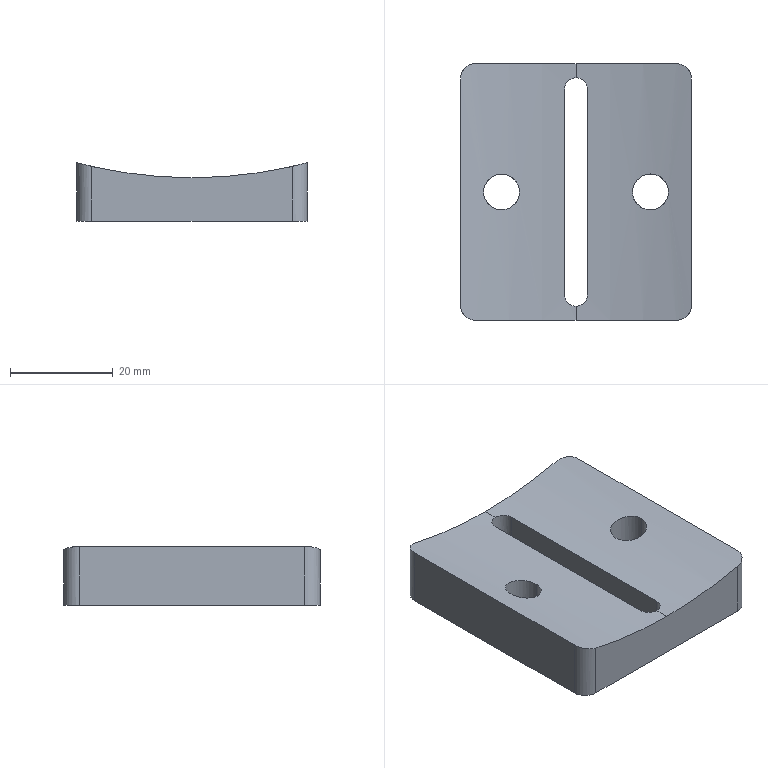Part | SolidWorks | features ICE 2, Extrusion 1, Fillet 1, HoleWzd 1 | 1 solid | 24 faces | box 45 x 50 x 11.442 mm | volume 18116 mm3 | cylinder 14 | plane 10 | commonest cylinder face diameters 6 x4 7 x4 4.5 x2 8 x2 175 x2
STEP:
#1=CARTESIAN_POINT('',(18.,25.,-85.629));
#2=VERTEX_POINT('',#1);
#3=CARTESIAN_POINT('',(11.,25.,-86.806));
#4=VERTEX_POINT('',#3);
#5=CARTESIAN_POINT('',(18.,25.,-85.629));
#6=CARTESIAN_POINT('',(18.,24.77,-85.629));
#7=CARTESIAN_POINT('',(17.978,24.541,-85.633));
#8=CARTESIAN_POINT('',(17.887,24.087,-85.652));
#9=CARTESIAN_POINT('',(17.819,23.865,-85.666));
#10=CARTESIAN_POINT('',(17.643,23.443,-85.703));
#11=CARTESIAN_POINT('',(17.533,23.239,-85.725));
#12=CARTESIAN_POINT('',(17.276,22.856,-85.778));
#13=CARTESIAN_POINT('',(17.131,22.681,-85.807));
#14=CARTESIAN_POINT('',(16.808,22.359,-85.871));
#15=CARTESIAN_POINT('',(16.628,22.212,-85.906));
#16=CARTESIAN_POINT('',(16.25,21.96,-85.978));
#17=CARTESIAN_POINT('',(16.05,21.854,-86.016));
#18=CARTESIAN_POINT('',(15.629,21.679,-86.093));
#19=CARTESIAN_POINT('',(15.409,21.612,-86.133));
#20=CARTESIAN_POINT('',(14.965,21.524,-86.211));
#21=CARTESIAN_POINT('',(14.739,21.501,-86.25));
#22=CARTESIAN_POINT('',(14.28,21.499,-86.327));
#23=CARTESIAN_POINT('',(14.054,21.521,-86.364));
#24=CARTESIAN_POINT('',(13.609,21.608,-86.436));
#25=CARTESIAN_POINT('',(13.388,21.674,-86.47));
#26=CARTESIAN_POINT('',(12.964,21.847,-86.535));
#27=CARTESIAN_POINT('',(12.763,21.953,-86.564));
#28=CARTESIAN_POINT('',(12.381,22.205,-86.62));
#29=CARTESIAN_POINT('',(12.2,22.352,-86.645));
#30=CARTESIAN_POINT('',(11.875,22.674,-86.691));
#31=CARTESIAN_POINT('',(11.729,22.85,-86.71));
#32=CARTESIAN_POINT('',(11.47,23.232,-86.745));
#33=CARTESIAN_POINT('',(11.36,23.437,-86.76));
#34=CARTESIAN_POINT('',(11.094,24.072,-86.794));
#35=CARTESIAN_POINT('',(11.,24.534,-86.806));
#36=CARTESIAN_POINT('',(11.,25.,-86.806));
#37=B_SPLINE_CURVE_WITH_KNOTS('',3,(#5,#6,#7,#8,#9,#10,#11,#12,#13,#14,#15,#16,#17,#18,#19,#20,#21,#22,#23,#24,#25,#26,#27,#28,#29,#30,#31,#32,#33,#34,#35,#36),.UNSPECIFIED.,.F.,.F.,(4,2,2,2,2,2,2,2,2,2,2,2,2,2,2,4),(0.01102,0.01171,0.0124,0.01309,0.01378,0.01447,0.01515,0.01584,0.01653,0.01722,0.01791,0.0186,0.01929,0.01997,0.02066,0.02204),.UNSPECIFIED.);
#38=EDGE_CURVE('',#2,#4,#37,.T.);
#39=ORIENTED_EDGE('',*,*,#38,.F.);
#40=CARTESIAN_POINT('',(18.,25.,-96.));
#41=VERTEX_POINT('',#40);
#42=CARTESIAN_POINT('',(18.,25.,-96.));
#43=DIRECTION('',(0.,0.,-1.));
#44=VECTOR('',#43,1000.);
#45=LINE('',#42,#44);
#46=EDGE_CURVE('',#2,#41,#45,.T.);
#47=ORIENTED_EDGE('',*,*,#46,.T.);
#48=CARTESIAN_POINT('',(11.,25.,-96.));
#49=VERTEX_POINT('',#48);
#50=CARTESIAN_POINT('',(14.5,25.,-96.));
#51=DIRECTION('',(0.,0.,-1.));
#52=DIRECTION('',(-1.,0.,0.));
#53=AXIS2_PLACEMENT_3D('',#50,#51,#52);
#54=CIRCLE('',#53,3.5);
#55=EDGE_CURVE('',#41,#49,#54,.T.);
#56=ORIENTED_EDGE('',*,*,#55,.T.);
#57=CARTESIAN_POINT('',(11.,25.,-96.));
#58=DIRECTION('',(0.,0.,-1.));
#59=VECTOR('',#58,1000.);
#60=LINE('',#57,#59);
#61=EDGE_CURVE('',#4,#49,#60,.T.);
#62=ORIENTED_EDGE('',*,*,#61,.F.);
#63=EDGE_LOOP('',(#39,#47,#56,#62));
#64=FACE_OUTER_BOUND('',#63,.T.);
#65=CARTESIAN_POINT('',(14.5,25.,-96.));
#66=DIRECTION('',(0.,0.,-1.));
#67=DIRECTION('',(-1.,0.,0.));
#68=AXIS2_PLACEMENT_3D('',#65,#66,#67);
#69=CYLINDRICAL_SURFACE('',#68,3.5);
#70=ADVANCED_FACE('',(#64),#69,.F.);
#71=CARTESIAN_POINT('',(-11.,25.,-86.806));
#72=VERTEX_POINT('',#71);
#73=CARTESIAN_POINT('',(-18.,25.,-85.629));
#74=VERTEX_POINT('',#73);
#75=CARTESIAN_POINT('',(-11.,25.,-86.806));
#76=CARTESIAN_POINT('',(-11.,24.77,-86.806));
#77=CARTESIAN_POINT('',(-11.022,24.541,-86.803));
#78=CARTESIAN_POINT('',(-11.113,24.087,-86.791));
#79=CARTESIAN_POINT('',(-11.181,23.865,-86.783));
#80=CARTESIAN_POINT('',(-11.358,23.441,-86.76));
#81=CARTESIAN_POINT('',(-11.468,23.237,-86.745));
#82=CARTESIAN_POINT('',(-11.726,22.854,-86.711));
#83=CARTESIAN_POINT('',(-11.872,22.677,-86.691));
#84=CARTESIAN_POINT('',(-12.197,22.355,-86.646));
#85=CARTESIAN_POINT('',(-12.378,22.207,-86.62));
#86=CARTESIAN_POINT('',(-12.759,21.955,-86.565));
#87=CARTESIAN_POINT('',(-12.96,21.849,-86.535));
#88=CARTESIAN_POINT('',(-13.384,21.675,-86.471));
#89=CARTESIAN_POINT('',(-13.605,21.609,-86.436));
#90=CARTESIAN_POINT('',(-14.051,21.522,-86.365));
#91=CARTESIAN_POINT('',(-14.277,21.5,-86.328));
#92=CARTESIAN_POINT('',(-14.736,21.5,-86.251));
#93=CARTESIAN_POINT('',(-14.961,21.523,-86.212));
#94=CARTESIAN_POINT('',(-15.405,21.612,-86.133));
#95=CARTESIAN_POINT('',(-15.626,21.678,-86.094));
#96=CARTESIAN_POINT('',(-16.047,21.852,-86.016));
#97=CARTESIAN_POINT('',(-16.247,21.959,-85.979));
#98=CARTESIAN_POINT('',(-16.625,22.21,-85.906));
#99=CARTESIAN_POINT('',(-16.805,22.357,-85.871));
#100=CARTESIAN_POINT('',(-17.128,22.678,-85.807));
#101=CARTESIAN_POINT('',(-17.274,22.853,-85.778));
#102=CARTESIAN_POINT('',(-17.531,23.234,-85.726));
#103=CARTESIAN_POINT('',(-17.641,23.439,-85.703));
#104=CARTESIAN_POINT('',(-17.906,24.072,-85.649));
#105=CARTESIAN_POINT('',(-18.,24.534,-85.629));
#106=CARTESIAN_POINT('',(-18.,25.,-85.629));
#107=B_SPLINE_CURVE_WITH_KNOTS('',3,(#75,#76,#77,#78,#79,#80,#81,#82,#83,#84,#85,#86,#87,#88,#89,#90,#91,#92,#93,#94,#95,#96,#97,#98,#99,#100,#101,#102,#103,#104,#105,#106),.UNSPECIFIED.,.F.,.F.,(4,2,2,2,2,2,2,2,2,2,2,2,2,2,2,4),(0.01102,0.01171,0.0124,0.01309,0.01378,0.01447,0.01515,0.01584,0.01653,0.01722,0.01791,0.0186,0.01929,0.01998,0.02066,0.02204),.UNSPECIFIED.);
#108=EDGE_CURVE('',#72,#74,#107,.T.);
#109=ORIENTED_EDGE('',*,*,#108,.F.);
#110=CARTESIAN_POINT('',(-11.,25.,-96.));
#111=VERTEX_POINT('',#110);
#112=CARTESIAN_POINT('',(-11.,25.,-96.));
#113=DIRECTION('',(0.,0.,-1.));
#114=VECTOR('',#113,1000.);
#115=LINE('',#112,#114);
#116=EDGE_CURVE('',#72,#111,#115,.T.);
#117=ORIENTED_EDGE('',*,*,#116,.T.);
#118=CARTESIAN_POINT('',(-18.,25.,-96.));
#119=VERTEX_POINT('',#118);
#120=CARTESIAN_POINT('',(-14.5,25.,-96.));
#121=DIRECTION('',(0.,0.,-1.));
#122=DIRECTION('',(-1.,0.,0.));
#123=AXIS2_PLACEMENT_3D('',#120,#121,#122);
#124=CIRCLE('',#123,3.5);
#125=EDGE_CURVE('',#111,#119,#124,.T.);
#126=ORIENTED_EDGE('',*,*,#125,.T.);
#127=CARTESIAN_POINT('',(-18.,25.,-96.));
#128=DIRECTION('',(0.,0.,-1.));
#129=VECTOR('',#128,1000.);
#130=LINE('',#127,#129);
#131=EDGE_CURVE('',#74,#119,#130,.T.);
#132=ORIENTED_EDGE('',*,*,#131,.F.);
#133=EDGE_LOOP('',(#109,#117,#126,#132));
#134=FACE_OUTER_BOUND('',#133,.T.);
#135=CARTESIAN_POINT('',(-14.5,25.,-96.));
#136=DIRECTION('',(0.,0.,-1.));
#137=DIRECTION('',(-1.,0.,0.));
#138=AXIS2_PLACEMENT_3D('',#135,#136,#137);
#139=CYLINDRICAL_SURFACE('',#138,3.5);
#140=ADVANCED_FACE('',(#134),#139,.F.);
#141=CARTESIAN_POINT('',(11.,25.,-86.806));
#142=CARTESIAN_POINT('',(11.,25.233,-86.806));
#143=CARTESIAN_POINT('',(11.023,25.462,-86.803));
#144=CARTESIAN_POINT('',(11.113,25.912,-86.791));
#145=CARTESIAN_POINT('',(11.181,26.136,-86.783));
#146=CARTESIAN_POINT('',(11.359,26.562,-86.76));
#147=CARTESIAN_POINT('',(11.468,26.764,-86.745));
#148=CARTESIAN_POINT('',(11.725,27.145,-86.711));
#149=CARTESIAN_POINT('',(11.874,27.325,-86.691));
#150=CARTESIAN_POINT('',(12.199,27.647,-86.646));
#151=CARTESIAN_POINT('',(12.376,27.792,-86.621));
#152=CARTESIAN_POINT('',(12.761,28.046,-86.565));
#153=CARTESIAN_POINT('',(12.964,28.153,-86.535));
#154=CARTESIAN_POINT('',(13.385,28.325,-86.47));
#155=CARTESIAN_POINT('',(13.606,28.392,-86.436));
#156=CARTESIAN_POINT('',(14.055,28.479,-86.364));
#157=CARTESIAN_POINT('',(14.281,28.5,-86.327));
#158=CARTESIAN_POINT('',(14.734,28.5,-86.251));
#159=CARTESIAN_POINT('',(14.965,28.476,-86.211));
#160=CARTESIAN_POINT('',(15.41,28.387,-86.133));
#161=CARTESIAN_POINT('',(15.626,28.322,-86.094));
#162=CARTESIAN_POINT('',(16.047,28.148,-86.016));
#163=CARTESIAN_POINT('',(16.251,28.039,-85.978));
#164=CARTESIAN_POINT('',(16.628,27.788,-85.906));
#165=CARTESIAN_POINT('',(16.805,27.644,-85.871));
#166=CARTESIAN_POINT('',(17.131,27.319,-85.807));
#167=CARTESIAN_POINT('',(17.277,27.143,-85.777));
#168=CARTESIAN_POINT('',(17.531,26.764,-85.726));
#169=CARTESIAN_POINT('',(17.642,26.56,-85.703));
#170=CARTESIAN_POINT('',(17.819,26.134,-85.666));
#171=CARTESIAN_POINT('',(17.886,25.915,-85.652));
#172=CARTESIAN_POINT('',(17.977,25.464,-85.633));
#173=CARTESIAN_POINT('',(18.,25.23,-85.629));
#174=CARTESIAN_POINT('',(18.,25.,-85.629));
#175=B_SPLINE_CURVE_WITH_KNOTS('',3,(#141,#142,#143,#144,#145,#146,#147,#148,#149,#150,#151,#152,#153,#154,#155,#156,#157,#158,#159,#160,#161,#162,#163,#164,#165,#166,#167,#168,#169,#170,#171,#172,#173,#174),.UNSPECIFIED.,.F.,.F.,(4,2,2,2,2,2,2,2,2,2,2,2,2,2,2,2,4),(0.,0.0006889,0.001378,0.002067,0.002756,0.003444,0.004133,0.004822,0.005511,0.0062,0.006889,0.007578,0.008267,0.008955,0.009644,0.01033,0.01102),.UNSPECIFIED.);
#176=EDGE_CURVE('',#4,#2,#175,.T.);
#177=ORIENTED_EDGE('',*,*,#176,.T.);
#178=ORIENTED_EDGE('',*,*,#38,.T.);
#179=EDGE_LOOP('',(#177,#178));
#180=FACE_BOUND('',#179,.T.);
#181=CARTESIAN_POINT('',(0.,50.,-87.5));
#182=VERTEX_POINT('',#181);
#183=CARTESIAN_POINT('',(19.5,50.,-85.299));
#184=VERTEX_POINT('',#183);
#185=CARTESIAN_POINT('',(0.,50.,0.));
#186=DIRECTION('',(0.,-1.,0.));
#187=DIRECTION('',(0.,0.,1.));
#188=AXIS2_PLACEMENT_3D('',#185,#186,#187);
#189=CIRCLE('',#188,87.5);
#190=EDGE_CURVE('',#182,#184,#189,.T.);
#191=ORIENTED_EDGE('',*,*,#190,.F.);
#192=CARTESIAN_POINT('',(0.,47.25,-87.5));
#193=VERTEX_POINT('',#192);
#194=CARTESIAN_POINT('',(0.,50.,-87.5));
#195=DIRECTION('',(0.,-1.,0.));
#196=VECTOR('',#195,1000.);
#197=LINE('',#194,#196);
#198=EDGE_CURVE('',#182,#193,#197,.T.);
#199=ORIENTED_EDGE('',*,*,#198,.T.);
#200=CARTESIAN_POINT('',(2.25,45.,-87.471));
#201=VERTEX_POINT('',#200);
#202=CARTESIAN_POINT('',(0.,47.25,-87.5));
#203=CARTESIAN_POINT('',(0.1467,47.25,-87.5));
#204=CARTESIAN_POINT('',(0.2956,47.235,-87.5));
#205=CARTESIAN_POINT('',(0.584,47.178,-87.498));
#206=CARTESIAN_POINT('',(0.7242,47.135,-87.497));
#207=CARTESIAN_POINT('',(0.9964,47.023,-87.494));
#208=CARTESIAN_POINT('',(1.128,46.952,-87.493));
#209=CARTESIAN_POINT('',(1.372,46.789,-87.489));
#210=CARTESIAN_POINT('',(1.485,46.697,-87.487));
#211=CARTESIAN_POINT('',(1.695,46.487,-87.484));
#212=CARTESIAN_POINT('',(1.789,46.373,-87.482));
#213=CARTESIAN_POINT('',(1.952,46.129,-87.478));
#214=CARTESIAN_POINT('',(2.022,45.998,-87.477));
#215=CARTESIAN_POINT('',(2.135,45.726,-87.474));
#216=CARTESIAN_POINT('',(2.177,45.585,-87.473));
#217=CARTESIAN_POINT('',(2.235,45.297,-87.471));
#218=CARTESIAN_POINT('',(2.25,45.149,-87.471));
#219=CARTESIAN_POINT('',(2.25,45.,-87.471));
#220=B_SPLINE_CURVE_WITH_KNOTS('',3,(#202,#203,#204,#205,#206,#207,#208,#209,#210,#211,#212,#213,#214,#215,#216,#217,#218,#219),.UNSPECIFIED.,.F.,.F.,(4,2,2,2,2,2,2,2,4),(0.003518,0.003958,0.004397,0.004836,0.005276,0.005715,0.006155,0.006594,0.007033),.UNSPECIFIED.);
#221=EDGE_CURVE('',#193,#201,#220,.T.);
#222=ORIENTED_EDGE('',*,*,#221,.T.);
#223=CARTESIAN_POINT('',(2.25,5.,-87.471));
#224=VERTEX_POINT('',#223);
#225=CARTESIAN_POINT('',(2.25,50.,-87.471));
#226=DIRECTION('',(0.,-1.,0.));
#227=VECTOR('',#226,1000.);
#228=LINE('',#225,#227);
#229=EDGE_CURVE('',#201,#224,#228,.T.);
#230=ORIENTED_EDGE('',*,*,#229,.T.);
#231=CARTESIAN_POINT('',(0.,2.75,-87.5));
#232=VERTEX_POINT('',#231);
#233=CARTESIAN_POINT('',(2.25,5.,-87.471));
#234=CARTESIAN_POINT('',(2.25,4.851,-87.471));
#235=CARTESIAN_POINT('',(2.235,4.705,-87.471));
#236=CARTESIAN_POINT('',(2.178,4.417,-87.473));
#237=CARTESIAN_POINT('',(2.135,4.274,-87.474));
#238=CARTESIAN_POINT('',(2.022,4.002,-87.477));
#239=CARTESIAN_POINT('',(1.953,3.873,-87.478));
#240=CARTESIAN_POINT('',(1.789,3.628,-87.482));
#241=CARTESIAN_POINT('',(1.694,3.512,-87.484));
#242=CARTESIAN_POINT('',(1.383,3.201,-87.489));
#243=CARTESIAN_POINT('',(1.132,3.033,-87.493));
#244=CARTESIAN_POINT('',(0.5898,2.809,-87.498));
#245=CARTESIAN_POINT('',(0.2936,2.75,-87.5));
#246=CARTESIAN_POINT('',(0.,2.75,-87.5));
#247=B_SPLINE_CURVE_WITH_KNOTS('',3,(#233,#234,#235,#236,#237,#238,#239,#240,#241,#242,#243,#244,#245,#246),.UNSPECIFIED.,.F.,.F.,(4,2,2,2,2,2,4),(0.,0.0004398,0.0008796,0.001319,0.001759,0.002639,0.003518),.UNSPECIFIED.);
#248=EDGE_CURVE('',#224,#232,#247,.T.);
#249=ORIENTED_EDGE('',*,*,#248,.T.);
#250=CARTESIAN_POINT('',(0.,0.,-87.5));
#251=VERTEX_POINT('',#250);
#252=CARTESIAN_POINT('',(0.,50.,-87.5));
#253=DIRECTION('',(0.,-1.,0.));
#254=VECTOR('',#253,1000.);
#255=LINE('',#252,#254);
#256=EDGE_CURVE('',#232,#251,#255,.T.);
#257=ORIENTED_EDGE('',*,*,#256,.T.);
#258=CARTESIAN_POINT('',(19.5,0.,-85.299));
#259=VERTEX_POINT('',#258);
#260=CARTESIAN_POINT('',(0.,0.,0.));
#261=DIRECTION('',(0.,-1.,0.));
#262=DIRECTION('',(0.,0.,1.));
#263=AXIS2_PLACEMENT_3D('',#260,#261,#262);
#264=CIRCLE('',#263,87.5);
#265=EDGE_CURVE('',#251,#259,#264,.T.);
#266=ORIENTED_EDGE('',*,*,#265,.T.);
#267=CARTESIAN_POINT('',(22.5,3.,-84.558));
#268=VERTEX_POINT('',#267);
#269=CARTESIAN_POINT('',(19.5,0.,-85.299));
#270=CARTESIAN_POINT('',(19.696,0.,-85.255));
#271=CARTESIAN_POINT('',(19.889,0.01901,-85.21));
#272=CARTESIAN_POINT('',(20.268,0.09343,-85.121));
#273=CARTESIAN_POINT('',(20.456,0.1496,-85.076));
#274=CARTESIAN_POINT('',(20.816,0.2972,-84.988));
#275=CARTESIAN_POINT('',(20.988,0.3876,-84.946));
#276=CARTESIAN_POINT('',(21.312,0.6014,-84.865));
#277=CARTESIAN_POINT('',(21.467,0.7264,-84.826));
#278=CARTESIAN_POINT('',(21.746,1.001,-84.755));
#279=CARTESIAN_POINT('',(21.871,1.151,-84.723));
#280=CARTESIAN_POINT('',(22.092,1.477,-84.665));
#281=CARTESIAN_POINT('',(22.188,1.654,-84.64));
#282=CARTESIAN_POINT('',(22.418,2.199,-84.58));
#283=CARTESIAN_POINT('',(22.5,2.598,-84.558));
#284=CARTESIAN_POINT('',(22.5,3.,-84.558));
#285=B_SPLINE_CURVE_WITH_KNOTS('',3,(#269,#270,#271,#272,#273,#274,#275,#276,#277,#278,#279,#280,#281,#282,#283,#284),.UNSPECIFIED.,.F.,.F.,(4,2,2,2,2,2,2,4),(0.,0.0005945,0.001189,0.001783,0.002378,0.002972,0.003567,0.004756),.UNSPECIFIED.);
#286=EDGE_CURVE('',#259,#268,#285,.T.);
#287=ORIENTED_EDGE('',*,*,#286,.T.);
#288=CARTESIAN_POINT('',(22.5,47.,-84.558));
#289=VERTEX_POINT('',#288);
#290=CARTESIAN_POINT('',(22.5,50.,-84.558));
#291=DIRECTION('',(0.,-1.,0.));
#292=VECTOR('',#291,1000.);
#293=LINE('',#290,#292);
#294=EDGE_CURVE('',#289,#268,#293,.T.);
#295=ORIENTED_EDGE('',*,*,#294,.F.);
#296=CARTESIAN_POINT('',(22.5,47.,-84.558));
#297=CARTESIAN_POINT('',(22.5,47.201,-84.558));
#298=CARTESIAN_POINT('',(22.48,47.399,-84.563));
#299=CARTESIAN_POINT('',(22.402,47.787,-84.584));
#300=CARTESIAN_POINT('',(22.342,47.98,-84.599));
#301=CARTESIAN_POINT('',(22.189,48.345,-84.64));
#302=CARTESIAN_POINT('',(22.095,48.518,-84.664));
#303=CARTESIAN_POINT('',(21.874,48.845,-84.722));
#304=CARTESIAN_POINT('',(21.747,48.998,-84.755));
#305=CARTESIAN_POINT('',(21.33,49.409,-84.861));
#306=CARTESIAN_POINT('',(20.996,49.629,-84.944));
#307=CARTESIAN_POINT('',(20.459,49.849,-85.075));
#308=CARTESIAN_POINT('',(20.271,49.906,-85.12));
#309=CARTESIAN_POINT('',(19.889,49.981,-85.21));
#310=CARTESIAN_POINT('',(19.696,50.,-85.255));
#311=CARTESIAN_POINT('',(19.5,50.,-85.299));
#312=B_SPLINE_CURVE_WITH_KNOTS('',3,(#296,#297,#298,#299,#300,#301,#302,#303,#304,#305,#306,#307,#308,#309,#310,#311),.UNSPECIFIED.,.F.,.F.,(4,2,2,2,2,2,2,4),(0.,0.0005945,0.001189,0.001783,0.002378,0.003567,0.004161,0.004756),.UNSPECIFIED.);
#313=EDGE_CURVE('',#289,#184,#312,.T.);
#314=ORIENTED_EDGE('',*,*,#313,.T.);
#315=EDGE_LOOP('',(#191,#199,#222,#230,#249,#257,#266,#287,#295,#314));
#316=FACE_OUTER_BOUND('',#315,.T.);
#317=CARTESIAN_POINT('',(0.,50.,0.));
#318=DIRECTION('',(0.,-1.,0.));
#319=DIRECTION('',(0.,0.,-1.));
#320=AXIS2_PLACEMENT_3D('',#317,#318,#319);
#321=CYLINDRICAL_SURFACE('',#320,87.5);
#322=ADVANCED_FACE('',(#180,#316),#321,.F.);
#323=CARTESIAN_POINT('',(2.25,45.,-92.));
#324=VERTEX_POINT('',#323);
#325=CARTESIAN_POINT('',(-2.25,45.,-92.));
#326=VERTEX_POINT('',#325);
#327=CARTESIAN_POINT('',(0.,45.,-92.));
#328=DIRECTION('',(0.,0.,1.));
#329=DIRECTION('',(-1.,0.,0.));
#330=AXIS2_PLACEMENT_3D('',#327,#328,#329);
#331=CIRCLE('',#330,2.25);
#332=EDGE_CURVE('',#324,#326,#331,.T.);
#333=ORIENTED_EDGE('',*,*,#332,.F.);
#334=CARTESIAN_POINT('',(2.25,45.,-84.558));
#335=DIRECTION('',(0.,0.,-1.));
#336=VECTOR('',#335,1000.);
#337=LINE('',#334,#336);
#338=EDGE_CURVE('',#201,#324,#337,.T.);
#339=ORIENTED_EDGE('',*,*,#338,.F.);
#340=ORIENTED_EDGE('',*,*,#221,.F.);
#341=CARTESIAN_POINT('',(-2.25,45.,-87.471));
#342=VERTEX_POINT('',#341);
#343=CARTESIAN_POINT('',(-2.25,45.,-87.471));
#344=CARTESIAN_POINT('',(-2.25,45.149,-87.471));
#345=CARTESIAN_POINT('',(-2.235,45.295,-87.471));
#346=CARTESIAN_POINT('',(-2.178,45.583,-87.473));
#347=CARTESIAN_POINT('',(-2.135,45.726,-87.474));
#348=CARTESIAN_POINT('',(-2.022,45.998,-87.477));
#349=CARTESIAN_POINT('',(-1.953,46.127,-87.478));
#350=CARTESIAN_POINT('',(-1.789,46.372,-87.482));
#351=CARTESIAN_POINT('',(-1.694,46.488,-87.484));
#352=CARTESIAN_POINT('',(-1.383,46.799,-87.489));
#353=CARTESIAN_POINT('',(-1.132,46.967,-87.493));
#354=CARTESIAN_POINT('',(-0.5898,47.191,-87.498));
#355=CARTESIAN_POINT('',(-0.2936,47.25,-87.5));
#356=CARTESIAN_POINT('',(0.,47.25,-87.5));
#357=B_SPLINE_CURVE_WITH_KNOTS('',3,(#343,#344,#345,#346,#347,#348,#349,#350,#351,#352,#353,#354,#355,#356),.UNSPECIFIED.,.F.,.F.,(4,2,2,2,2,2,4),(0.,0.0004398,0.0008796,0.001319,0.001759,0.002639,0.003518),.UNSPECIFIED.);
#358=EDGE_CURVE('',#342,#193,#357,.T.);
#359=ORIENTED_EDGE('',*,*,#358,.F.);
#360=CARTESIAN_POINT('',(-2.25,45.,-84.558));
#361=DIRECTION('',(0.,0.,-1.));
#362=VECTOR('',#361,1000.);
#363=LINE('',#360,#362);
#364=EDGE_CURVE('',#342,#326,#363,.T.);
#365=ORIENTED_EDGE('',*,*,#364,.T.);
#366=EDGE_LOOP('',(#333,#339,#340,#359,#365));
#367=FACE_OUTER_BOUND('',#366,.T.);
#368=CARTESIAN_POINT('',(0.,45.,-84.558));
#369=DIRECTION('',(0.,0.,-1.));
#370=DIRECTION('',(-1.,0.,0.));
#371=AXIS2_PLACEMENT_3D('',#368,#369,#370);
#372=CYLINDRICAL_SURFACE('',#371,2.25);
#373=ADVANCED_FACE('',(#367),#372,.F.);
#374=CARTESIAN_POINT('',(-2.25,5.,-92.));
#375=VERTEX_POINT('',#374);
#376=CARTESIAN_POINT('',(-2.25,45.,-92.));
#377=DIRECTION('',(0.,-1.,0.));
#378=VECTOR('',#377,1000.);
#379=LINE('',#376,#378);
#380=EDGE_CURVE('',#326,#375,#379,.T.);
#381=ORIENTED_EDGE('',*,*,#380,.F.);
#382=ORIENTED_EDGE('',*,*,#364,.F.);
#383=CARTESIAN_POINT('',(-2.25,5.,-87.471));
#384=VERTEX_POINT('',#383);
#385=CARTESIAN_POINT('',(-2.25,50.,-87.471));
#386=DIRECTION('',(0.,1.,0.));
#387=VECTOR('',#386,1000.);
#388=LINE('',#385,#387);
#389=EDGE_CURVE('',#384,#342,#388,.T.);
#390=ORIENTED_EDGE('',*,*,#389,.F.);
#391=CARTESIAN_POINT('',(-2.25,5.,-84.558));
#392=DIRECTION('',(0.,0.,-1.));
#393=VECTOR('',#392,1000.);
#394=LINE('',#391,#393);
#395=EDGE_CURVE('',#384,#375,#394,.T.);
#396=ORIENTED_EDGE('',*,*,#395,.T.);
#397=EDGE_LOOP('',(#381,#382,#390,#396));
#398=FACE_OUTER_BOUND('',#397,.T.);
#399=CARTESIAN_POINT('',(-2.25,45.,-84.558));
#400=DIRECTION('',(-1.,0.,0.));
#401=DIRECTION('',(0.,0.,1.));
#402=AXIS2_PLACEMENT_3D('',#399,#400,#401);
#403=PLANE('',#402);
#404=ADVANCED_FACE('',(#398),#403,.F.);
#405=CARTESIAN_POINT('',(2.25,5.,-92.));
#406=VERTEX_POINT('',#405);
#407=CARTESIAN_POINT('',(0.,5.,-92.));
#408=DIRECTION('',(0.,0.,1.));
#409=DIRECTION('',(-1.,0.,0.));
#410=AXIS2_PLACEMENT_3D('',#407,#408,#409);
#411=CIRCLE('',#410,2.25);
#412=EDGE_CURVE('',#375,#406,#411,.T.);
#413=ORIENTED_EDGE('',*,*,#412,.F.);
#414=ORIENTED_EDGE('',*,*,#395,.F.);
#415=CARTESIAN_POINT('',(0.,2.75,-87.5));
#416=CARTESIAN_POINT('',(-0.1467,2.75,-87.5));
#417=CARTESIAN_POINT('',(-0.2956,2.765,-87.5));
#418=CARTESIAN_POINT('',(-0.584,2.822,-87.498));
#419=CARTESIAN_POINT('',(-0.7242,2.865,-87.497));
#420=CARTESIAN_POINT('',(-0.9964,2.977,-87.494));
#421=CARTESIAN_POINT('',(-1.128,3.048,-87.493));
#422=CARTESIAN_POINT('',(-1.372,3.211,-87.489));
#423=CARTESIAN_POINT('',(-1.485,3.303,-87.487));
#424=CARTESIAN_POINT('',(-1.695,3.513,-87.484));
#425=CARTESIAN_POINT('',(-1.789,3.627,-87.482));
#426=CARTESIAN_POINT('',(-1.952,3.871,-87.478));
#427=CARTESIAN_POINT('',(-2.022,4.002,-87.477));
#428=CARTESIAN_POINT('',(-2.135,4.274,-87.474));
#429=CARTESIAN_POINT('',(-2.177,4.415,-87.473));
#430=CARTESIAN_POINT('',(-2.235,4.703,-87.471));
#431=CARTESIAN_POINT('',(-2.25,4.851,-87.471));
#432=CARTESIAN_POINT('',(-2.25,5.,-87.471));
#433=B_SPLINE_CURVE_WITH_KNOTS('',3,(#415,#416,#417,#418,#419,#420,#421,#422,#423,#424,#425,#426,#427,#428,#429,#430,#431,#432),.UNSPECIFIED.,.F.,.F.,(4,2,2,2,2,2,2,2,4),(0.003518,0.003958,0.004397,0.004836,0.005276,0.005715,0.006155,0.006594,0.007033),.UNSPECIFIED.);
#434=EDGE_CURVE('',#232,#384,#433,.T.);
#435=ORIENTED_EDGE('',*,*,#434,.F.);
#436=ORIENTED_EDGE('',*,*,#248,.F.);
#437=CARTESIAN_POINT('',(2.25,5.,-84.558));
#438=DIRECTION('',(0.,0.,-1.));
#439=VECTOR('',#438,1000.);
#440=LINE('',#437,#439);
#441=EDGE_CURVE('',#224,#406,#440,.T.);
#442=ORIENTED_EDGE('',*,*,#441,.T.);
#443=EDGE_LOOP('',(#413,#414,#435,#436,#442));
#444=FACE_OUTER_BOUND('',#443,.T.);
#445=CARTESIAN_POINT('',(0.,5.,-84.558));
#446=DIRECTION('',(0.,0.,-1.));
#447=DIRECTION('',(-1.,0.,0.));
#448=AXIS2_PLACEMENT_3D('',#445,#446,#447);
#449=CYLINDRICAL_SURFACE('',#448,2.25);
#450=ADVANCED_FACE('',(#444),#449,.F.);
#451=CARTESIAN_POINT('',(2.25,45.,-92.));
#452=DIRECTION('',(0.,1.,0.));
#453=VECTOR('',#452,1000.);
#454=LINE('',#451,#453);
#455=EDGE_CURVE('',#406,#324,#454,.T.);
#456=ORIENTED_EDGE('',*,*,#455,.F.);
#457=ORIENTED_EDGE('',*,*,#441,.F.);
#458=ORIENTED_EDGE('',*,*,#229,.F.);
#459=ORIENTED_EDGE('',*,*,#338,.T.);
#460=EDGE_LOOP('',(#456,#457,#458,#459));
#461=FACE_OUTER_BOUND('',#460,.T.);
#462=CARTESIAN_POINT('',(2.25,45.,-84.558));
#463=DIRECTION('',(1.,0.,0.));
#464=DIRECTION('',(0.,0.,-1.));
#465=AXIS2_PLACEMENT_3D('',#462,#463,#464);
#466=PLANE('',#465);
#467=ADVANCED_FACE('',(#461),#466,.F.);
#468=CARTESIAN_POINT('',(4.,45.,-96.));
#469=VERTEX_POINT('',#468);
#470=CARTESIAN_POINT('',(4.,5.,-96.));
#471=VERTEX_POINT('',#470);
#472=CARTESIAN_POINT('',(4.,45.,-96.));
#473=DIRECTION('',(0.,-1.,0.));
#474=VECTOR('',#473,1000.);
#475=LINE('',#472,#474);
#476=EDGE_CURVE('',#469,#471,#475,.T.);
#477=ORIENTED_EDGE('',*,*,#476,.F.);
#478=CARTESIAN_POINT('',(-4.,45.,-96.));
#479=VERTEX_POINT('',#478);
#480=CARTESIAN_POINT('',(0.,45.,-96.));
#481=DIRECTION('',(0.,0.,-1.));
#482=DIRECTION('',(-1.,0.,0.));
#483=AXIS2_PLACEMENT_3D('',#480,#481,#482);
#484=CIRCLE('',#483,4.);
#485=EDGE_CURVE('',#479,#469,#484,.T.);
#486=ORIENTED_EDGE('',*,*,#485,.F.);
#487=CARTESIAN_POINT('',(-4.,5.,-96.));
#488=VERTEX_POINT('',#487);
#489=CARTESIAN_POINT('',(-4.,45.,-96.));
#490=DIRECTION('',(0.,1.,0.));
#491=VECTOR('',#490,1000.);
#492=LINE('',#489,#491);
#493=EDGE_CURVE('',#488,#479,#492,.T.);
#494=ORIENTED_EDGE('',*,*,#493,.F.);
#495=CARTESIAN_POINT('',(0.,5.,-96.));
#496=DIRECTION('',(0.,0.,-1.));
#497=DIRECTION('',(-1.,0.,0.));
#498=AXIS2_PLACEMENT_3D('',#495,#496,#497);
#499=CIRCLE('',#498,4.);
#500=EDGE_CURVE('',#471,#488,#499,.T.);
#501=ORIENTED_EDGE('',*,*,#500,.F.);
#502=EDGE_LOOP('',(#477,#486,#494,#501));
#503=FACE_BOUND('',#502,.T.);
#504=CARTESIAN_POINT('',(14.5,25.,-96.));
#505=DIRECTION('',(0.,0.,-1.));
#506=DIRECTION('',(-1.,0.,0.));
#507=AXIS2_PLACEMENT_3D('',#504,#505,#506);
#508=CIRCLE('',#507,3.5);
#509=EDGE_CURVE('',#49,#41,#508,.T.);
#510=ORIENTED_EDGE('',*,*,#509,.F.);
#511=ORIENTED_EDGE('',*,*,#55,.F.);
#512=EDGE_LOOP('',(#510,#511));
#513=FACE_BOUND('',#512,.T.);
#514=CARTESIAN_POINT('',(-14.5,25.,-96.));
#515=DIRECTION('',(0.,0.,-1.));
#516=DIRECTION('',(-1.,0.,0.));
#517=AXIS2_PLACEMENT_3D('',#514,#515,#516);
#518=CIRCLE('',#517,3.5);
#519=EDGE_CURVE('',#119,#111,#518,.T.);
#520=ORIENTED_EDGE('',*,*,#519,.F.);
#521=ORIENTED_EDGE('',*,*,#125,.F.);
#522=EDGE_LOOP('',(#520,#521));
#523=FACE_BOUND('',#522,.T.);
#524=CARTESIAN_POINT('',(-22.5,47.,-96.));
#525=VERTEX_POINT('',#524);
#526=CARTESIAN_POINT('',(-22.5,3.,-96.));
#527=VERTEX_POINT('',#526);
#528=CARTESIAN_POINT('',(-22.5,50.,-96.));
#529=DIRECTION('',(0.,-1.,0.));
#530=VECTOR('',#529,1000.);
#531=LINE('',#528,#530);
#532=EDGE_CURVE('',#525,#527,#531,.T.);
#533=ORIENTED_EDGE('',*,*,#532,.F.);
#534=CARTESIAN_POINT('',(-19.5,50.,-96.));
#535=VERTEX_POINT('',#534);
#536=CARTESIAN_POINT('',(-19.5,47.,-96.));
#537=DIRECTION('',(0.,0.,-1.));
#538=DIRECTION('',(1.,0.,0.));
#539=AXIS2_PLACEMENT_3D('',#536,#537,#538);
#540=CIRCLE('',#539,3.);
#541=EDGE_CURVE('',#525,#535,#540,.T.);
#542=ORIENTED_EDGE('',*,*,#541,.T.);
#543=CARTESIAN_POINT('',(19.5,50.,-96.));
#544=VERTEX_POINT('',#543);
#545=CARTESIAN_POINT('',(-22.5,50.,-96.));
#546=DIRECTION('',(-1.,0.,0.));
#547=VECTOR('',#546,1000.);
#548=LINE('',#545,#547);
#549=EDGE_CURVE('',#544,#535,#548,.T.);
#550=ORIENTED_EDGE('',*,*,#549,.F.);
#551=CARTESIAN_POINT('',(22.5,47.,-96.));
#552=VERTEX_POINT('',#551);
#553=CARTESIAN_POINT('',(19.5,47.,-96.));
#554=DIRECTION('',(0.,0.,-1.));
#555=DIRECTION('',(1.,0.,0.));
#556=AXIS2_PLACEMENT_3D('',#553,#554,#555);
#557=CIRCLE('',#556,3.);
#558=EDGE_CURVE('',#544,#552,#557,.T.);
#559=ORIENTED_EDGE('',*,*,#558,.T.);
#560=CARTESIAN_POINT('',(22.5,3.,-96.));
#561=VERTEX_POINT('',#560);
#562=CARTESIAN_POINT('',(22.5,50.,-96.));
#563=DIRECTION('',(0.,-1.,0.));
#564=VECTOR('',#563,1000.);
#565=LINE('',#562,#564);
#566=EDGE_CURVE('',#552,#561,#565,.T.);
#567=ORIENTED_EDGE('',*,*,#566,.T.);
#568=CARTESIAN_POINT('',(19.5,0.,-96.));
#569=VERTEX_POINT('',#568);
#570=CARTESIAN_POINT('',(19.5,3.,-96.));
#571=DIRECTION('',(0.,0.,-1.));
#572=DIRECTION('',(1.,0.,0.));
#573=AXIS2_PLACEMENT_3D('',#570,#571,#572);
#574=CIRCLE('',#573,3.);
#575=EDGE_CURVE('',#561,#569,#574,.T.);
#576=ORIENTED_EDGE('',*,*,#575,.T.);
#577=CARTESIAN_POINT('',(-19.5,0.,-96.));
#578=VERTEX_POINT('',#577);
#579=CARTESIAN_POINT('',(-22.5,0.,-96.));
#580=DIRECTION('',(-1.,0.,0.));
#581=VECTOR('',#580,1000.);
#582=LINE('',#579,#581);
#583=EDGE_CURVE('',#569,#578,#582,.T.);
#584=ORIENTED_EDGE('',*,*,#583,.T.);
#585=CARTESIAN_POINT('',(-19.5,3.,-96.));
#586=DIRECTION('',(0.,0.,-1.));
#587=DIRECTION('',(1.,0.,0.));
#588=AXIS2_PLACEMENT_3D('',#585,#586,#587);
#589=CIRCLE('',#588,3.);
#590=EDGE_CURVE('',#578,#527,#589,.T.);
#591=ORIENTED_EDGE('',*,*,#590,.T.);
#592=EDGE_LOOP('',(#533,#542,#550,#559,#567,#576,#584,#591));
#593=FACE_OUTER_BOUND('',#592,.T.);
#594=CARTESIAN_POINT('',(-22.5,50.,-96.));
#595=DIRECTION('',(0.,0.,1.));
#596=DIRECTION('',(1.,0.,0.));
#597=AXIS2_PLACEMENT_3D('',#594,#595,#596);
#598=PLANE('',#597);
#599=ADVANCED_FACE('',(#503,#513,#523,#593),#598,.F.);
#600=CARTESIAN_POINT('',(-22.5,47.,-84.558));
#601=VERTEX_POINT('',#600);
#602=CARTESIAN_POINT('',(-22.5,3.,-84.558));
#603=VERTEX_POINT('',#602);
#604=CARTESIAN_POINT('',(-22.5,50.,-84.558));
#605=DIRECTION('',(0.,-1.,0.));
#606=VECTOR('',#605,1000.);
#607=LINE('',#604,#606);
#608=EDGE_CURVE('',#601,#603,#607,.T.);
#609=ORIENTED_EDGE('',*,*,#608,.F.);
#610=CARTESIAN_POINT('',(-22.5,47.,-96.));
#611=DIRECTION('',(0.,0.,-1.));
#612=VECTOR('',#611,1000.);
#613=LINE('',#610,#612);
#614=EDGE_CURVE('',#601,#525,#613,.T.);
#615=ORIENTED_EDGE('',*,*,#614,.T.);
#616=ORIENTED_EDGE('',*,*,#532,.T.);
#617=CARTESIAN_POINT('',(-22.5,3.,-84.558));
#618=DIRECTION('',(0.,0.,1.));
#619=VECTOR('',#618,1000.);
#620=LINE('',#617,#619);
#621=EDGE_CURVE('',#527,#603,#620,.T.);
#622=ORIENTED_EDGE('',*,*,#621,.T.);
#623=EDGE_LOOP('',(#609,#615,#616,#622));
#624=FACE_OUTER_BOUND('',#623,.T.);
#625=CARTESIAN_POINT('',(-22.5,50.,-84.558));
#626=DIRECTION('',(1.,0.,0.));
#627=DIRECTION('',(0.,0.,-1.));
#628=AXIS2_PLACEMENT_3D('',#625,#626,#627);
#629=PLANE('',#628);
#630=ADVANCED_FACE('',(#624),#629,.F.);
#631=ORIENTED_EDGE('',*,*,#198,.F.);
#632=CARTESIAN_POINT('',(-19.5,50.,-85.299));
#633=VERTEX_POINT('',#632);
#634=CARTESIAN_POINT('',(0.,50.,0.));
#635=DIRECTION('',(0.,-1.,0.));
#636=DIRECTION('',(0.,0.,1.));
#637=AXIS2_PLACEMENT_3D('',#634,#635,#636);
#638=CIRCLE('',#637,87.5);
#639=EDGE_CURVE('',#633,#182,#638,.T.);
#640=ORIENTED_EDGE('',*,*,#639,.F.);
#641=CARTESIAN_POINT('',(-19.5,50.,-85.299));
#642=CARTESIAN_POINT('',(-19.696,50.,-85.255));
#643=CARTESIAN_POINT('',(-19.889,49.981,-85.21));
#644=CARTESIAN_POINT('',(-20.268,49.907,-85.121));
#645=CARTESIAN_POINT('',(-20.456,49.85,-85.076));
#646=CARTESIAN_POINT('',(-20.816,49.703,-84.988));
#647=CARTESIAN_POINT('',(-20.988,49.612,-84.946));
#648=CARTESIAN_POINT('',(-21.312,49.399,-84.865));
#649=CARTESIAN_POINT('',(-21.467,49.274,-84.826));
#650=CARTESIAN_POINT('',(-21.746,48.999,-84.755));
#651=CARTESIAN_POINT('',(-21.871,48.849,-84.723));
#652=CARTESIAN_POINT('',(-22.092,48.523,-84.665));
#653=CARTESIAN_POINT('',(-22.188,48.346,-84.64));
#654=CARTESIAN_POINT('',(-22.418,47.801,-84.58));
#655=CARTESIAN_POINT('',(-22.5,47.402,-84.558));
#656=CARTESIAN_POINT('',(-22.5,47.,-84.558));
#657=B_SPLINE_CURVE_WITH_KNOTS('',3,(#641,#642,#643,#644,#645,#646,#647,#648,#649,#650,#651,#652,#653,#654,#655,#656),.UNSPECIFIED.,.F.,.F.,(4,2,2,2,2,2,2,4),(0.,0.0005945,0.001189,0.001783,0.002378,0.002972,0.003567,0.004756),.UNSPECIFIED.);
#658=EDGE_CURVE('',#633,#601,#657,.T.);
#659=ORIENTED_EDGE('',*,*,#658,.T.);
#660=ORIENTED_EDGE('',*,*,#608,.T.);
#661=CARTESIAN_POINT('',(-19.5,0.,-85.299));
#662=VERTEX_POINT('',#661);
#663=CARTESIAN_POINT('',(-22.5,3.,-84.558));
#664=CARTESIAN_POINT('',(-22.5,2.799,-84.558));
#665=CARTESIAN_POINT('',(-22.48,2.601,-84.563));
#666=CARTESIAN_POINT('',(-22.402,2.213,-84.584));
#667=CARTESIAN_POINT('',(-22.342,2.02,-84.599));
#668=CARTESIAN_POINT('',(-22.189,1.655,-84.64));
#669=CARTESIAN_POINT('',(-22.095,1.482,-84.664));
#670=CARTESIAN_POINT('',(-21.874,1.155,-84.722));
#671=CARTESIAN_POINT('',(-21.747,1.002,-84.755));
#672=CARTESIAN_POINT('',(-21.33,0.5909,-84.861));
#673=CARTESIAN_POINT('',(-20.996,0.3712,-84.944));
#674=CARTESIAN_POINT('',(-20.459,0.151,-85.075));
#675=CARTESIAN_POINT('',(-20.271,0.09433,-85.12));
#676=CARTESIAN_POINT('',(-19.889,0.019,-85.21));
#677=CARTESIAN_POINT('',(-19.696,0.,-85.255));
#678=CARTESIAN_POINT('',(-19.5,0.,-85.299));
#679=B_SPLINE_CURVE_WITH_KNOTS('',3,(#663,#664,#665,#666,#667,#668,#669,#670,#671,#672,#673,#674,#675,#676,#677,#678),.UNSPECIFIED.,.F.,.F.,(4,2,2,2,2,2,2,4),(0.,0.0005945,0.001189,0.001783,0.002378,0.003567,0.004161,0.004756),.UNSPECIFIED.);
#680=EDGE_CURVE('',#603,#662,#679,.T.);
#681=ORIENTED_EDGE('',*,*,#680,.T.);
#682=CARTESIAN_POINT('',(0.,0.,0.));
#683=DIRECTION('',(0.,-1.,0.));
#684=DIRECTION('',(0.,0.,1.));
#685=AXIS2_PLACEMENT_3D('',#682,#683,#684);
#686=CIRCLE('',#685,87.5);
#687=EDGE_CURVE('',#662,#251,#686,.T.);
#688=ORIENTED_EDGE('',*,*,#687,.T.);
#689=ORIENTED_EDGE('',*,*,#256,.F.);
#690=ORIENTED_EDGE('',*,*,#434,.T.);
#691=ORIENTED_EDGE('',*,*,#389,.T.);
#692=ORIENTED_EDGE('',*,*,#358,.T.);
#693=EDGE_LOOP('',(#631,#640,#659,#660,#681,#688,#689,#690,#691,#692));
#694=FACE_OUTER_BOUND('',#693,.T.);
#695=CARTESIAN_POINT('',(-18.,25.,-85.629));
#696=CARTESIAN_POINT('',(-18.,25.233,-85.629));
#697=CARTESIAN_POINT('',(-17.977,25.462,-85.633));
#698=CARTESIAN_POINT('',(-17.887,25.912,-85.652));
#699=CARTESIAN_POINT('',(-17.819,26.136,-85.667));
#700=CARTESIAN_POINT('',(-17.641,26.561,-85.703));
#701=CARTESIAN_POINT('',(-17.533,26.762,-85.726));
#702=CARTESIAN_POINT('',(-17.277,27.142,-85.777));
#703=CARTESIAN_POINT('',(-17.129,27.322,-85.807));
#704=CARTESIAN_POINT('',(-16.806,27.643,-85.871));
#705=CARTESIAN_POINT('',(-16.63,27.787,-85.905));
#706=CARTESIAN_POINT('',(-16.248,28.041,-85.978));
#707=CARTESIAN_POINT('',(-16.046,28.148,-86.016));
#708=CARTESIAN_POINT('',(-15.628,28.321,-86.093));
#709=CARTESIAN_POINT('',(-15.408,28.388,-86.133));
#710=CARTESIAN_POINT('',(-14.961,28.477,-86.212));
#711=CARTESIAN_POINT('',(-14.735,28.499,-86.251));
#712=CARTESIAN_POINT('',(-14.282,28.501,-86.327));
#713=CARTESIAN_POINT('',(-14.051,28.479,-86.365));
#714=CARTESIAN_POINT('',(-13.605,28.391,-86.436));
#715=CARTESIAN_POINT('',(-13.387,28.326,-86.47));
#716=CARTESIAN_POINT('',(-12.964,28.153,-86.535));
#717=CARTESIAN_POINT('',(-12.759,28.045,-86.565));
#718=CARTESIAN_POINT('',(-12.378,27.793,-86.62));
#719=CARTESIAN_POINT('',(-12.201,27.649,-86.645));
#720=CARTESIAN_POINT('',(-11.872,27.323,-86.691));
#721=CARTESIAN_POINT('',(-11.726,27.146,-86.711));
#722=CARTESIAN_POINT('',(-11.47,26.766,-86.745));
#723=CARTESIAN_POINT('',(-11.359,26.561,-86.76));
#724=CARTESIAN_POINT('',(-11.181,26.135,-86.783));
#725=CARTESIAN_POINT('',(-11.114,25.915,-86.791));
#726=CARTESIAN_POINT('',(-11.023,25.464,-86.803));
#727=CARTESIAN_POINT('',(-11.,25.23,-86.806));
#728=CARTESIAN_POINT('',(-11.,25.,-86.806));
#729=B_SPLINE_CURVE_WITH_KNOTS('',3,(#695,#696,#697,#698,#699,#700,#701,#702,#703,#704,#705,#706,#707,#708,#709,#710,#711,#712,#713,#714,#715,#716,#717,#718,#719,#720,#721,#722,#723,#724,#725,#726,#727,#728),.UNSPECIFIED.,.F.,.F.,(4,2,2,2,2,2,2,2,2,2,2,2,2,2,2,2,4),(0.,0.0006889,0.001378,0.002067,0.002755,0.003444,0.004133,0.004822,0.005511,0.0062,0.006889,0.007578,0.008266,0.008955,0.009644,0.01033,0.01102),.UNSPECIFIED.);
#730=EDGE_CURVE('',#74,#72,#729,.T.);
#731=ORIENTED_EDGE('',*,*,#730,.T.);
#732=ORIENTED_EDGE('',*,*,#108,.T.);
#733=EDGE_LOOP('',(#731,#732));
#734=FACE_BOUND('',#733,.T.);
#735=CARTESIAN_POINT('',(0.,50.,0.));
#736=DIRECTION('',(0.,-1.,0.));
#737=DIRECTION('',(0.,0.,-1.));
#738=AXIS2_PLACEMENT_3D('',#735,#736,#737);
#739=CYLINDRICAL_SURFACE('',#738,87.5);
#740=ADVANCED_FACE('',(#694,#734),#739,.F.);
#741=ORIENTED_EDGE('',*,*,#566,.F.);
#742=CARTESIAN_POINT('',(22.5,47.,-84.558));
#743=DIRECTION('',(0.,0.,1.));
#744=VECTOR('',#743,1000.);
#745=LINE('',#742,#744);
#746=EDGE_CURVE('',#552,#289,#745,.T.);
#747=ORIENTED_EDGE('',*,*,#746,.T.);
#748=ORIENTED_EDGE('',*,*,#294,.T.);
#749=CARTESIAN_POINT('',(22.5,3.,-96.));
#750=DIRECTION('',(0.,0.,-1.));
#751=VECTOR('',#750,1000.);
#752=LINE('',#749,#751);
#753=EDGE_CURVE('',#268,#561,#752,.T.);
#754=ORIENTED_EDGE('',*,*,#753,.T.);
#755=EDGE_LOOP('',(#741,#747,#748,#754));
#756=FACE_OUTER_BOUND('',#755,.T.);
#757=CARTESIAN_POINT('',(22.5,50.,-96.));
#758=DIRECTION('',(-1.,0.,0.));
#759=DIRECTION('',(0.,0.,1.));
#760=AXIS2_PLACEMENT_3D('',#757,#758,#759);
#761=PLANE('',#760);
#762=ADVANCED_FACE('',(#756),#761,.F.);
#763=ORIENTED_EDGE('',*,*,#549,.T.);
#764=CARTESIAN_POINT('',(-19.5,50.,-84.558));
#765=DIRECTION('',(0.,0.,1.));
#766=VECTOR('',#765,1000.);
#767=LINE('',#764,#766);
#768=EDGE_CURVE('',#535,#633,#767,.T.);
#769=ORIENTED_EDGE('',*,*,#768,.T.);
#770=ORIENTED_EDGE('',*,*,#639,.T.);
#771=ORIENTED_EDGE('',*,*,#190,.T.);
#772=CARTESIAN_POINT('',(19.5,50.,-96.));
#773=DIRECTION('',(0.,0.,-1.));
#774=VECTOR('',#773,1000.);
#775=LINE('',#772,#774);
#776=EDGE_CURVE('',#184,#544,#775,.T.);
#777=ORIENTED_EDGE('',*,*,#776,.T.);
#778=EDGE_LOOP('',(#763,#769,#770,#771,#777));
#779=FACE_OUTER_BOUND('',#778,.T.);
#780=CARTESIAN_POINT('',(0.,50.,0.));
#781=DIRECTION('',(0.,1.,0.));
#782=DIRECTION('',(0.,0.,1.));
#783=AXIS2_PLACEMENT_3D('',#780,#781,#782);
#784=PLANE('',#783);
#785=ADVANCED_FACE('',(#779),#784,.T.);
#786=ORIENTED_EDGE('',*,*,#687,.F.);
#787=CARTESIAN_POINT('',(-19.5,0.,0.));
#788=DIRECTION('',(0.,0.,-1.));
#789=VECTOR('',#788,1000.);
#790=LINE('',#787,#789);
#791=EDGE_CURVE('',#662,#578,#790,.T.);
#792=ORIENTED_EDGE('',*,*,#791,.T.);
#793=ORIENTED_EDGE('',*,*,#583,.F.);
#794=CARTESIAN_POINT('',(19.5,0.,0.));
#795=DIRECTION('',(0.,0.,1.));
#796=VECTOR('',#795,1000.);
#797=LINE('',#794,#796);
#798=EDGE_CURVE('',#569,#259,#797,.T.);
#799=ORIENTED_EDGE('',*,*,#798,.T.);
#800=ORIENTED_EDGE('',*,*,#265,.F.);
#801=EDGE_LOOP('',(#786,#792,#793,#799,#800));
#802=FACE_OUTER_BOUND('',#801,.T.);
#803=CARTESIAN_POINT('',(0.,0.,0.));
#804=DIRECTION('',(0.,1.,0.));
#805=DIRECTION('',(0.,0.,1.));
#806=AXIS2_PLACEMENT_3D('',#803,#804,#805);
#807=PLANE('',#806);
#808=ADVANCED_FACE('',(#802),#807,.F.);
#809=ORIENTED_EDGE('',*,*,#116,.F.);
#810=ORIENTED_EDGE('',*,*,#730,.F.);
#811=ORIENTED_EDGE('',*,*,#131,.T.);
#812=ORIENTED_EDGE('',*,*,#519,.T.);
#813=EDGE_LOOP('',(#809,#810,#811,#812));
#814=FACE_OUTER_BOUND('',#813,.T.);
#815=CARTESIAN_POINT('',(-14.5,25.,-96.));
#816=DIRECTION('',(0.,0.,-1.));
#817=DIRECTION('',(-1.,0.,0.));
#818=AXIS2_PLACEMENT_3D('',#815,#816,#817);
#819=CYLINDRICAL_SURFACE('',#818,3.5);
#820=ADVANCED_FACE('',(#814),#819,.F.);
#821=ORIENTED_EDGE('',*,*,#46,.F.);
#822=ORIENTED_EDGE('',*,*,#176,.F.);
#823=ORIENTED_EDGE('',*,*,#61,.T.);
#824=ORIENTED_EDGE('',*,*,#509,.T.);
#825=EDGE_LOOP('',(#821,#822,#823,#824));
#826=FACE_OUTER_BOUND('',#825,.T.);
#827=CARTESIAN_POINT('',(14.5,25.,-96.));
#828=DIRECTION('',(0.,0.,-1.));
#829=DIRECTION('',(-1.,0.,0.));
#830=AXIS2_PLACEMENT_3D('',#827,#828,#829);
#831=CYLINDRICAL_SURFACE('',#830,3.5);
#832=ADVANCED_FACE('',(#826),#831,.F.);
#833=CARTESIAN_POINT('',(-4.,45.,-92.));
#834=VERTEX_POINT('',#833);
#835=CARTESIAN_POINT('',(4.,45.,-92.));
#836=VERTEX_POINT('',#835);
#837=CARTESIAN_POINT('',(0.,45.,-92.));
#838=DIRECTION('',(0.,0.,-1.));
#839=DIRECTION('',(-1.,0.,0.));
#840=AXIS2_PLACEMENT_3D('',#837,#838,#839);
#841=CIRCLE('',#840,4.);
#842=EDGE_CURVE('',#834,#836,#841,.T.);
#843=ORIENTED_EDGE('',*,*,#842,.T.);
#844=CARTESIAN_POINT('',(4.,5.,-92.));
#845=VERTEX_POINT('',#844);
#846=CARTESIAN_POINT('',(4.,45.,-92.));
#847=DIRECTION('',(0.,-1.,0.));
#848=VECTOR('',#847,1000.);
#849=LINE('',#846,#848);
#850=EDGE_CURVE('',#836,#845,#849,.T.);
#851=ORIENTED_EDGE('',*,*,#850,.T.);
#852=CARTESIAN_POINT('',(-4.,5.,-92.));
#853=VERTEX_POINT('',#852);
#854=CARTESIAN_POINT('',(0.,5.,-92.));
#855=DIRECTION('',(0.,0.,-1.));
#856=DIRECTION('',(-1.,0.,0.));
#857=AXIS2_PLACEMENT_3D('',#854,#855,#856);
#858=CIRCLE('',#857,4.);
#859=EDGE_CURVE('',#845,#853,#858,.T.);
#860=ORIENTED_EDGE('',*,*,#859,.T.);
#861=CARTESIAN_POINT('',(-4.,45.,-92.));
#862=DIRECTION('',(0.,1.,0.));
#863=VECTOR('',#862,1000.);
#864=LINE('',#861,#863);
#865=EDGE_CURVE('',#853,#834,#864,.T.);
#866=ORIENTED_EDGE('',*,*,#865,.T.);
#867=EDGE_LOOP('',(#843,#851,#860,#866));
#868=FACE_OUTER_BOUND('',#867,.T.);
#869=ORIENTED_EDGE('',*,*,#332,.T.);
#870=ORIENTED_EDGE('',*,*,#380,.T.);
#871=ORIENTED_EDGE('',*,*,#412,.T.);
#872=ORIENTED_EDGE('',*,*,#455,.T.);
#873=EDGE_LOOP('',(#869,#870,#871,#872));
#874=FACE_BOUND('',#873,.T.);
#875=CARTESIAN_POINT('',(0.,45.,-92.));
#876=DIRECTION('',(0.,0.,-1.));
#877=DIRECTION('',(-1.,0.,0.));
#878=AXIS2_PLACEMENT_3D('',#875,#876,#877);
#879=PLANE('',#878);
#880=ADVANCED_FACE('',(#868,#874),#879,.T.);
#881=ORIENTED_EDGE('',*,*,#485,.T.);
#882=CARTESIAN_POINT('',(4.,45.,-92.));
#883=DIRECTION('',(0.,0.,-1.));
#884=VECTOR('',#883,1000.);
#885=LINE('',#882,#884);
#886=EDGE_CURVE('',#836,#469,#885,.T.);
#887=ORIENTED_EDGE('',*,*,#886,.F.);
#888=ORIENTED_EDGE('',*,*,#842,.F.);
#889=CARTESIAN_POINT('',(-4.,45.,-92.));
#890=DIRECTION('',(0.,0.,-1.));
#891=VECTOR('',#890,1000.);
#892=LINE('',#889,#891);
#893=EDGE_CURVE('',#834,#479,#892,.T.);
#894=ORIENTED_EDGE('',*,*,#893,.T.);
#895=EDGE_LOOP('',(#881,#887,#888,#894));
#896=FACE_OUTER_BOUND('',#895,.T.);
#897=CARTESIAN_POINT('',(0.,45.,-92.));
#898=DIRECTION('',(0.,0.,-1.));
#899=DIRECTION('',(-1.,0.,0.));
#900=AXIS2_PLACEMENT_3D('',#897,#898,#899);
#901=CYLINDRICAL_SURFACE('',#900,4.);
#902=ADVANCED_FACE('',(#896),#901,.F.);
#903=ORIENTED_EDGE('',*,*,#493,.T.);
#904=ORIENTED_EDGE('',*,*,#893,.F.);
#905=ORIENTED_EDGE('',*,*,#865,.F.);
#906=CARTESIAN_POINT('',(-4.,5.,-92.));
#907=DIRECTION('',(0.,0.,-1.));
#908=VECTOR('',#907,1000.);
#909=LINE('',#906,#908);
#910=EDGE_CURVE('',#853,#488,#909,.T.);
#911=ORIENTED_EDGE('',*,*,#910,.T.);
#912=EDGE_LOOP('',(#903,#904,#905,#911));
#913=FACE_OUTER_BOUND('',#912,.T.);
#914=CARTESIAN_POINT('',(-4.,45.,-92.));
#915=DIRECTION('',(-1.,0.,0.));
#916=DIRECTION('',(0.,-1.,0.));
#917=AXIS2_PLACEMENT_3D('',#914,#915,#916);
#918=PLANE('',#917);
#919=ADVANCED_FACE('',(#913),#918,.F.);
#920=ORIENTED_EDGE('',*,*,#500,.T.);
#921=ORIENTED_EDGE('',*,*,#910,.F.);
#922=ORIENTED_EDGE('',*,*,#859,.F.);
#923=CARTESIAN_POINT('',(4.,5.,-92.));
#924=DIRECTION('',(0.,0.,-1.));
#925=VECTOR('',#924,1000.);
#926=LINE('',#923,#925);
#927=EDGE_CURVE('',#845,#471,#926,.T.);
#928=ORIENTED_EDGE('',*,*,#927,.T.);
#929=EDGE_LOOP('',(#920,#921,#922,#928));
#930=FACE_OUTER_BOUND('',#929,.T.);
#931=CARTESIAN_POINT('',(0.,5.,-92.));
#932=DIRECTION('',(0.,0.,-1.));
#933=DIRECTION('',(-1.,0.,0.));
#934=AXIS2_PLACEMENT_3D('',#931,#932,#933);
#935=CYLINDRICAL_SURFACE('',#934,4.);
#936=ADVANCED_FACE('',(#930),#935,.F.);
#937=ORIENTED_EDGE('',*,*,#476,.T.);
#938=ORIENTED_EDGE('',*,*,#927,.F.);
#939=ORIENTED_EDGE('',*,*,#850,.F.);
#940=ORIENTED_EDGE('',*,*,#886,.T.);
#941=EDGE_LOOP('',(#937,#938,#939,#940));
#942=FACE_OUTER_BOUND('',#941,.T.);
#943=CARTESIAN_POINT('',(4.,45.,-92.));
#944=DIRECTION('',(1.,0.,0.));
#945=DIRECTION('',(0.,1.,0.));
#946=AXIS2_PLACEMENT_3D('',#943,#944,#945);
#947=PLANE('',#946);
#948=ADVANCED_FACE('',(#942),#947,.F.);
#949=ORIENTED_EDGE('',*,*,#541,.F.);
#950=ORIENTED_EDGE('',*,*,#614,.F.);
#951=ORIENTED_EDGE('',*,*,#658,.F.);
#952=ORIENTED_EDGE('',*,*,#768,.F.);
#953=EDGE_LOOP('',(#949,#950,#951,#952));
#954=FACE_OUTER_BOUND('',#953,.T.);
#955=CARTESIAN_POINT('',(-19.5,47.,0.));
#956=DIRECTION('',(0.,0.,-1.));
#957=DIRECTION('',(-1.,0.,0.));
#958=AXIS2_PLACEMENT_3D('',#955,#956,#957);
#959=CYLINDRICAL_SURFACE('',#958,3.);
#960=ADVANCED_FACE('',(#954),#959,.T.);
#961=ORIENTED_EDGE('',*,*,#313,.F.);
#962=ORIENTED_EDGE('',*,*,#746,.F.);
#963=ORIENTED_EDGE('',*,*,#558,.F.);
#964=ORIENTED_EDGE('',*,*,#776,.F.);
#965=EDGE_LOOP('',(#961,#962,#963,#964));
#966=FACE_OUTER_BOUND('',#965,.T.);
#967=CARTESIAN_POINT('',(19.5,47.,0.));
#968=DIRECTION('',(0.,0.,1.));
#969=DIRECTION('',(1.,0.,0.));
#970=AXIS2_PLACEMENT_3D('',#967,#968,#969);
#971=CYLINDRICAL_SURFACE('',#970,3.);
#972=ADVANCED_FACE('',(#966),#971,.T.);
#973=ORIENTED_EDGE('',*,*,#590,.F.);
#974=ORIENTED_EDGE('',*,*,#791,.F.);
#975=ORIENTED_EDGE('',*,*,#680,.F.);
#976=ORIENTED_EDGE('',*,*,#621,.F.);
#977=EDGE_LOOP('',(#973,#974,#975,#976));
#978=FACE_OUTER_BOUND('',#977,.T.);
#979=CARTESIAN_POINT('',(-19.5,3.,-84.558));
#980=DIRECTION('',(0.,0.,1.));
#981=DIRECTION('',(1.,0.,0.));
#982=AXIS2_PLACEMENT_3D('',#979,#980,#981);
#983=CYLINDRICAL_SURFACE('',#982,3.);
#984=ADVANCED_FACE('',(#978),#983,.T.);
#985=ORIENTED_EDGE('',*,*,#286,.F.);
#986=ORIENTED_EDGE('',*,*,#798,.F.);
#987=ORIENTED_EDGE('',*,*,#575,.F.);
#988=ORIENTED_EDGE('',*,*,#753,.F.);
#989=EDGE_LOOP('',(#985,#986,#987,#988));
#990=FACE_OUTER_BOUND('',#989,.T.);
#991=CARTESIAN_POINT('',(19.5,3.,-96.));
#992=DIRECTION('',(0.,0.,-1.));
#993=DIRECTION('',(-1.,0.,0.));
#994=AXIS2_PLACEMENT_3D('',#991,#992,#993);
#995=CYLINDRICAL_SURFACE('',#994,3.);
#996=ADVANCED_FACE('',(#990),#995,.T.);
#997=CLOSED_SHELL('',(#70,#140,#322,#373,#404,#450,#467,#599,#630,#740,#762,#785,#808,#820,#832,#880,#902,#919,#936,#948,#960,#972,#984,#996));
#998=MANIFOLD_SOLID_BREP('',#997);
#999=CARTESIAN_POINT('',(0.,0.,0.));
#1000=DIRECTION('',(0.,0.,1.));
#1001=DIRECTION('',(1.,0.,0.));
#1002=AXIS2_PLACEMENT_3D('',#999,#1000,#1001);
#1003=(LENGTH_UNIT()NAMED_UNIT(*)SI_UNIT(.MILLI.,.METRE.));
#1004=UNCERTAINTY_MEASURE_WITH_UNIT(LENGTH_MEASURE(0.00001),#1003,'','');
#1005=(NAMED_UNIT(*)PLANE_ANGLE_UNIT()SI_UNIT($,.RADIAN.));
#1006=(NAMED_UNIT(*)SI_UNIT($,.STERADIAN.)SOLID_ANGLE_UNIT());
#1007=(GEOMETRIC_REPRESENTATION_CONTEXT(3)GLOBAL_UNCERTAINTY_ASSIGNED_CONTEXT((#1004))GLOBAL_UNIT_ASSIGNED_CONTEXT((#1003,#1005,#1006))REPRESENTATION_CONTEXT('',''));
#1008=ADVANCED_BREP_SHAPE_REPRESENTATION('',(#998,#1002),#1007);